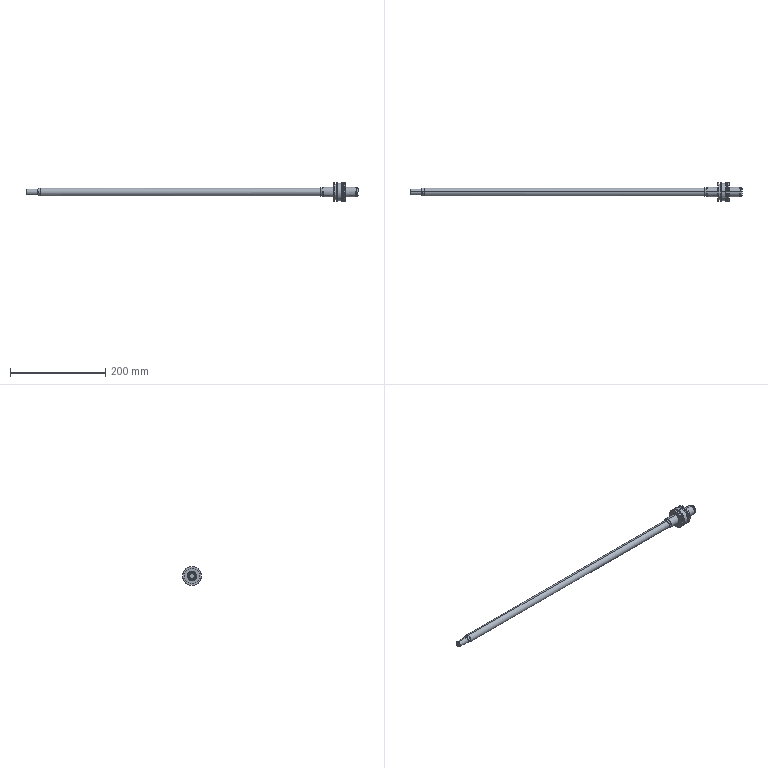Part | STEP file | SI_40x550-2 | 1 solid | 82 faces | box 695.5 x 39.5 x 39.5 mm | volume 154171 mm3 | cone 26 | cylinder 24 | plane 20 | spline 12 | commonest cylinder face diameters 39.5 x8 20 x4 32 x4 12 x2 16 x2 16.5 x2